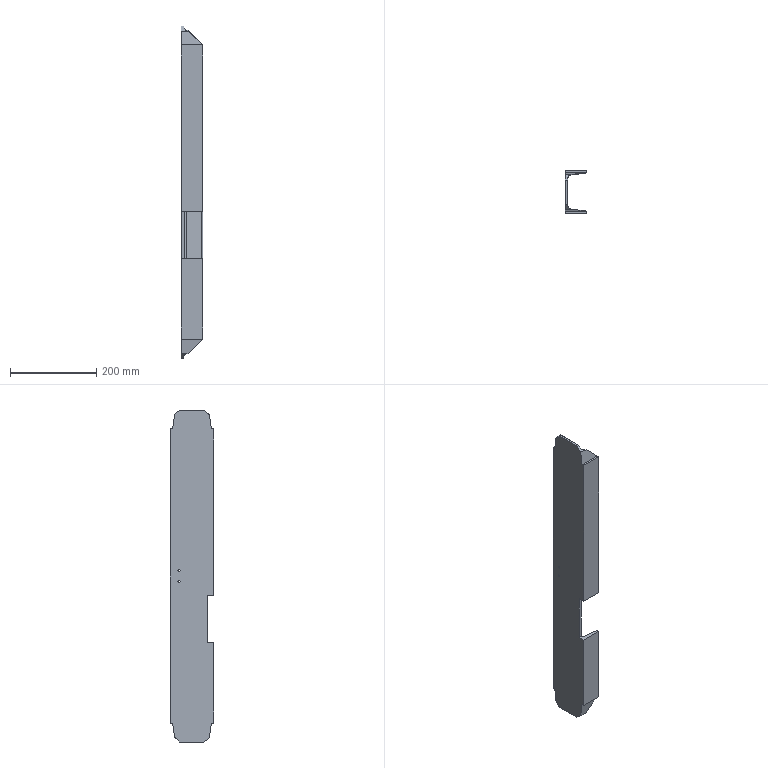Part | SolidWorks | features ICE 4, HoleWzd 2, Chamfer 1, Extrusion 1 | 1 solid | 53 faces | box 50 x 100 x 770 mm | volume 903448 mm3 | plane 28 | cylinder 25 | commonest cylinder face diameters 8.5 x16 5 x4 9 x3 17 x2